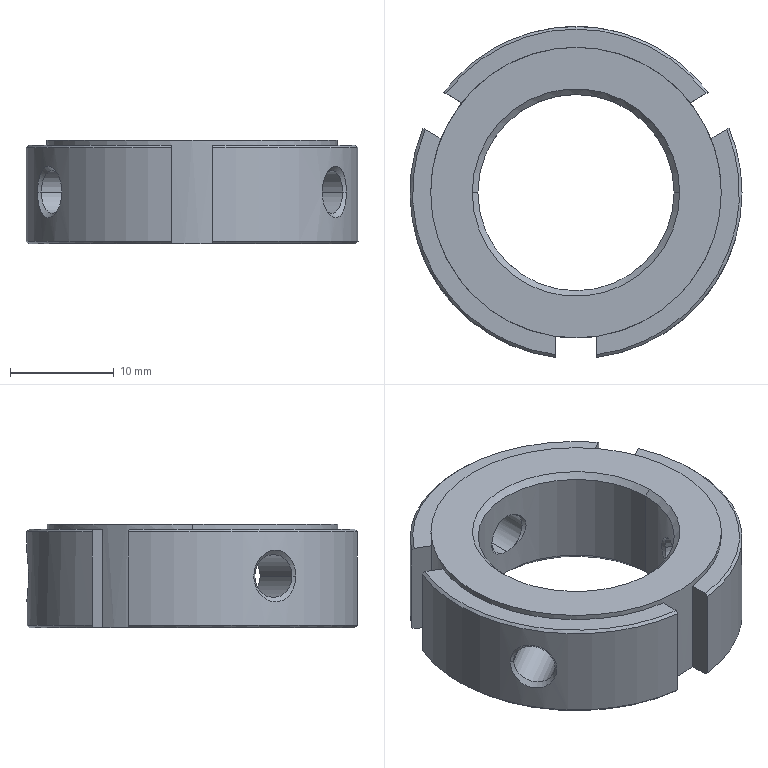Part | SolidWorks | features BaseBody 1 | 1 solid | 51 faces | box 32 x 31.875 x 10 mm | volume 4618 mm3 | cone 26 | cylinder 14 | plane 11 | commonest cylinder face diameters 4.134 x6 32 x4 18.917 x2 28 x2